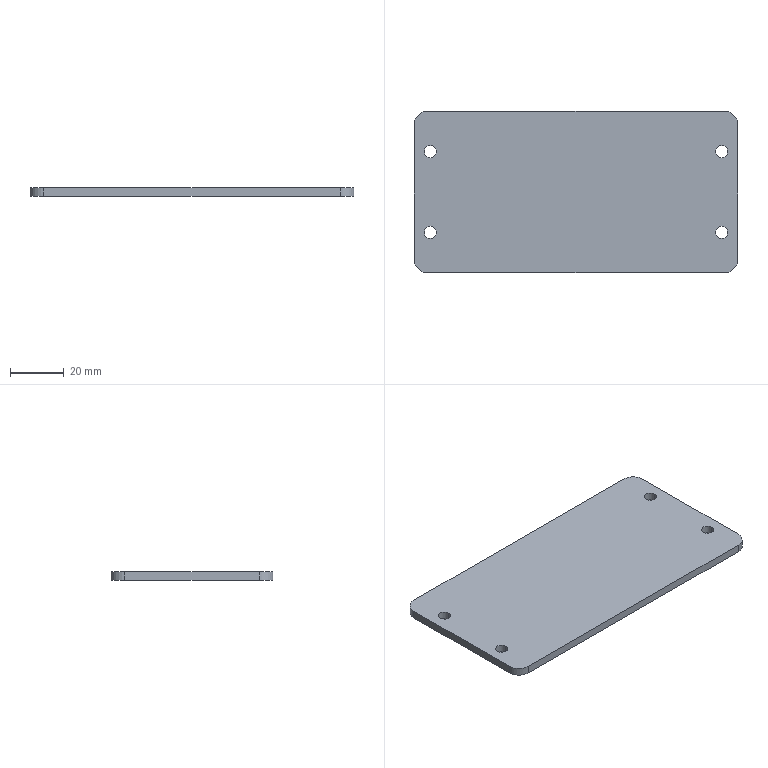Part | STEP file | 03-24 side guard plate | 1 solid | 18 faces | box 120 x 60 x 3 mm | volume 21345 mm3 | cylinder 12 | plane 6 | commonest cylinder face diameters 4.5 x8 10 x4
STEP:
#1=CARTESIAN_POINT('',(51.75,-15.,0.));
#2=VERTEX_POINT('',#1);
#3=CARTESIAN_POINT('',(56.25,-15.,0.));
#4=VERTEX_POINT('',#3);
#5=CARTESIAN_POINT('',(54.,-15.,0.));
#6=DIRECTION('',(0.,0.,1.));
#7=DIRECTION('',(1.,0.,0.));
#8=AXIS2_PLACEMENT_3D('',#5,#6,#7);
#9=CIRCLE('',#8,2.25);
#10=EDGE_CURVE('',#2,#4,#9,.T.);
#11=ORIENTED_EDGE('',*,*,#10,.F.);
#12=CARTESIAN_POINT('',(51.75,-15.,3.));
#13=VERTEX_POINT('',#12);
#14=CARTESIAN_POINT('',(51.75,-15.,-2.));
#15=DIRECTION('',(0.,0.,1.));
#16=VECTOR('',#15,1000.);
#17=LINE('',#14,#16);
#18=EDGE_CURVE('',#2,#13,#17,.T.);
#19=ORIENTED_EDGE('',*,*,#18,.T.);
#20=CARTESIAN_POINT('',(56.25,-15.,3.));
#21=VERTEX_POINT('',#20);
#22=CARTESIAN_POINT('',(54.,-15.,3.));
#23=DIRECTION('',(0.,0.,1.));
#24=DIRECTION('',(-1.,0.,0.));
#25=AXIS2_PLACEMENT_3D('',#22,#23,#24);
#26=CIRCLE('',#25,2.25);
#27=EDGE_CURVE('',#13,#21,#26,.T.);
#28=ORIENTED_EDGE('',*,*,#27,.T.);
#29=CARTESIAN_POINT('',(56.25,-15.,-2.));
#30=DIRECTION('',(0.,0.,1.));
#31=VECTOR('',#30,1000.);
#32=LINE('',#29,#31);
#33=EDGE_CURVE('',#4,#21,#32,.T.);
#34=ORIENTED_EDGE('',*,*,#33,.F.);
#35=EDGE_LOOP('',(#11,#19,#28,#34));
#36=FACE_OUTER_BOUND('',#35,.T.);
#37=CARTESIAN_POINT('',(54.,-15.,-2.));
#38=DIRECTION('',(0.,0.,1.));
#39=DIRECTION('',(1.,0.,0.));
#40=AXIS2_PLACEMENT_3D('',#37,#38,#39);
#41=CYLINDRICAL_SURFACE('',#40,2.25);
#42=ADVANCED_FACE('',(#36),#41,.F.);
#43=CARTESIAN_POINT('',(-56.25,15.,0.));
#44=VERTEX_POINT('',#43);
#45=CARTESIAN_POINT('',(-51.75,15.,0.));
#46=VERTEX_POINT('',#45);
#47=CARTESIAN_POINT('',(-54.,15.,0.));
#48=DIRECTION('',(0.,0.,1.));
#49=DIRECTION('',(1.,0.,0.));
#50=AXIS2_PLACEMENT_3D('',#47,#48,#49);
#51=CIRCLE('',#50,2.25);
#52=EDGE_CURVE('',#44,#46,#51,.T.);
#53=ORIENTED_EDGE('',*,*,#52,.F.);
#54=CARTESIAN_POINT('',(-56.25,15.,3.));
#55=VERTEX_POINT('',#54);
#56=CARTESIAN_POINT('',(-56.25,15.,-2.));
#57=DIRECTION('',(0.,0.,1.));
#58=VECTOR('',#57,1000.);
#59=LINE('',#56,#58);
#60=EDGE_CURVE('',#44,#55,#59,.T.);
#61=ORIENTED_EDGE('',*,*,#60,.T.);
#62=CARTESIAN_POINT('',(-51.75,15.,3.));
#63=VERTEX_POINT('',#62);
#64=CARTESIAN_POINT('',(-54.,15.,3.));
#65=DIRECTION('',(0.,0.,1.));
#66=DIRECTION('',(-1.,0.,0.));
#67=AXIS2_PLACEMENT_3D('',#64,#65,#66);
#68=CIRCLE('',#67,2.25);
#69=EDGE_CURVE('',#55,#63,#68,.T.);
#70=ORIENTED_EDGE('',*,*,#69,.T.);
#71=CARTESIAN_POINT('',(-51.75,15.,-2.));
#72=DIRECTION('',(0.,0.,1.));
#73=VECTOR('',#72,1000.);
#74=LINE('',#71,#73);
#75=EDGE_CURVE('',#46,#63,#74,.T.);
#76=ORIENTED_EDGE('',*,*,#75,.F.);
#77=EDGE_LOOP('',(#53,#61,#70,#76));
#78=FACE_OUTER_BOUND('',#77,.T.);
#79=CARTESIAN_POINT('',(-54.,15.,-2.));
#80=DIRECTION('',(0.,0.,1.));
#81=DIRECTION('',(1.,0.,0.));
#82=AXIS2_PLACEMENT_3D('',#79,#80,#81);
#83=CYLINDRICAL_SURFACE('',#82,2.25);
#84=ADVANCED_FACE('',(#78),#83,.F.);
#85=CARTESIAN_POINT('',(-56.25,-15.,0.));
#86=VERTEX_POINT('',#85);
#87=CARTESIAN_POINT('',(-51.75,-15.,0.));
#88=VERTEX_POINT('',#87);
#89=CARTESIAN_POINT('',(-54.,-15.,0.));
#90=DIRECTION('',(0.,0.,1.));
#91=DIRECTION('',(1.,0.,0.));
#92=AXIS2_PLACEMENT_3D('',#89,#90,#91);
#93=CIRCLE('',#92,2.25);
#94=EDGE_CURVE('',#86,#88,#93,.T.);
#95=ORIENTED_EDGE('',*,*,#94,.F.);
#96=CARTESIAN_POINT('',(-56.25,-15.,3.));
#97=VERTEX_POINT('',#96);
#98=CARTESIAN_POINT('',(-56.25,-15.,-2.));
#99=DIRECTION('',(0.,0.,1.));
#100=VECTOR('',#99,1000.);
#101=LINE('',#98,#100);
#102=EDGE_CURVE('',#86,#97,#101,.T.);
#103=ORIENTED_EDGE('',*,*,#102,.T.);
#104=CARTESIAN_POINT('',(-51.75,-15.,3.));
#105=VERTEX_POINT('',#104);
#106=CARTESIAN_POINT('',(-54.,-15.,3.));
#107=DIRECTION('',(0.,0.,1.));
#108=DIRECTION('',(1.,0.,0.));
#109=AXIS2_PLACEMENT_3D('',#106,#107,#108);
#110=CIRCLE('',#109,2.25);
#111=EDGE_CURVE('',#97,#105,#110,.T.);
#112=ORIENTED_EDGE('',*,*,#111,.T.);
#113=CARTESIAN_POINT('',(-51.75,-15.,-2.));
#114=DIRECTION('',(0.,0.,1.));
#115=VECTOR('',#114,1000.);
#116=LINE('',#113,#115);
#117=EDGE_CURVE('',#88,#105,#116,.T.);
#118=ORIENTED_EDGE('',*,*,#117,.F.);
#119=EDGE_LOOP('',(#95,#103,#112,#118));
#120=FACE_OUTER_BOUND('',#119,.T.);
#121=CARTESIAN_POINT('',(-54.,-15.,-2.));
#122=DIRECTION('',(0.,0.,1.));
#123=DIRECTION('',(1.,0.,0.));
#124=AXIS2_PLACEMENT_3D('',#121,#122,#123);
#125=CYLINDRICAL_SURFACE('',#124,2.25);
#126=ADVANCED_FACE('',(#120),#125,.F.);
#127=CARTESIAN_POINT('',(51.75,15.,0.));
#128=VERTEX_POINT('',#127);
#129=CARTESIAN_POINT('',(56.25,15.,0.));
#130=VERTEX_POINT('',#129);
#131=CARTESIAN_POINT('',(54.,15.,0.));
#132=DIRECTION('',(0.,0.,1.));
#133=DIRECTION('',(1.,0.,0.));
#134=AXIS2_PLACEMENT_3D('',#131,#132,#133);
#135=CIRCLE('',#134,2.25);
#136=EDGE_CURVE('',#128,#130,#135,.T.);
#137=ORIENTED_EDGE('',*,*,#136,.F.);
#138=CARTESIAN_POINT('',(51.75,15.,3.));
#139=VERTEX_POINT('',#138);
#140=CARTESIAN_POINT('',(51.75,15.,-2.));
#141=DIRECTION('',(0.,0.,1.));
#142=VECTOR('',#141,1000.);
#143=LINE('',#140,#142);
#144=EDGE_CURVE('',#128,#139,#143,.T.);
#145=ORIENTED_EDGE('',*,*,#144,.T.);
#146=CARTESIAN_POINT('',(56.25,15.,3.));
#147=VERTEX_POINT('',#146);
#148=CARTESIAN_POINT('',(54.,15.,3.));
#149=DIRECTION('',(0.,0.,1.));
#150=DIRECTION('',(1.,0.,0.));
#151=AXIS2_PLACEMENT_3D('',#148,#149,#150);
#152=CIRCLE('',#151,2.25);
#153=EDGE_CURVE('',#139,#147,#152,.T.);
#154=ORIENTED_EDGE('',*,*,#153,.T.);
#155=CARTESIAN_POINT('',(56.25,15.,-2.));
#156=DIRECTION('',(0.,0.,1.));
#157=VECTOR('',#156,1000.);
#158=LINE('',#155,#157);
#159=EDGE_CURVE('',#130,#147,#158,.T.);
#160=ORIENTED_EDGE('',*,*,#159,.F.);
#161=EDGE_LOOP('',(#137,#145,#154,#160));
#162=FACE_OUTER_BOUND('',#161,.T.);
#163=CARTESIAN_POINT('',(54.,15.,-2.));
#164=DIRECTION('',(0.,0.,1.));
#165=DIRECTION('',(1.,0.,0.));
#166=AXIS2_PLACEMENT_3D('',#163,#164,#165);
#167=CYLINDRICAL_SURFACE('',#166,2.25);
#168=ADVANCED_FACE('',(#162),#167,.F.);
#169=CARTESIAN_POINT('',(60.,-25.,3.));
#170=VERTEX_POINT('',#169);
#171=CARTESIAN_POINT('',(60.,25.,3.));
#172=VERTEX_POINT('',#171);
#173=CARTESIAN_POINT('',(60.,30.,3.));
#174=DIRECTION('',(0.,1.,0.));
#175=VECTOR('',#174,1000.);
#176=LINE('',#173,#175);
#177=EDGE_CURVE('',#170,#172,#176,.T.);
#178=ORIENTED_EDGE('',*,*,#177,.F.);
#179=CARTESIAN_POINT('',(60.,-25.,0.));
#180=VERTEX_POINT('',#179);
#181=CARTESIAN_POINT('',(60.,-25.,3.));
#182=DIRECTION('',(0.,0.,-1.));
#183=VECTOR('',#182,1000.);
#184=LINE('',#181,#183);
#185=EDGE_CURVE('',#170,#180,#184,.T.);
#186=ORIENTED_EDGE('',*,*,#185,.T.);
#187=CARTESIAN_POINT('',(60.,25.,0.));
#188=VERTEX_POINT('',#187);
#189=CARTESIAN_POINT('',(60.,30.,0.));
#190=DIRECTION('',(0.,1.,0.));
#191=VECTOR('',#190,1000.);
#192=LINE('',#189,#191);
#193=EDGE_CURVE('',#180,#188,#192,.T.);
#194=ORIENTED_EDGE('',*,*,#193,.T.);
#195=CARTESIAN_POINT('',(60.,25.,3.));
#196=DIRECTION('',(0.,0.,1.));
#197=VECTOR('',#196,1000.);
#198=LINE('',#195,#197);
#199=EDGE_CURVE('',#188,#172,#198,.T.);
#200=ORIENTED_EDGE('',*,*,#199,.T.);
#201=EDGE_LOOP('',(#178,#186,#194,#200));
#202=FACE_OUTER_BOUND('',#201,.T.);
#203=CARTESIAN_POINT('',(60.,30.,3.));
#204=DIRECTION('',(-1.,0.,0.));
#205=DIRECTION('',(0.,-1.,0.));
#206=AXIS2_PLACEMENT_3D('',#203,#204,#205);
#207=PLANE('',#206);
#208=ADVANCED_FACE('',(#202),#207,.F.);
#209=CARTESIAN_POINT('',(55.,30.,3.));
#210=VERTEX_POINT('',#209);
#211=CARTESIAN_POINT('',(-55.,30.,3.));
#212=VERTEX_POINT('',#211);
#213=CARTESIAN_POINT('',(-60.,30.,3.));
#214=DIRECTION('',(-1.,0.,0.));
#215=VECTOR('',#214,1000.);
#216=LINE('',#213,#215);
#217=EDGE_CURVE('',#210,#212,#216,.T.);
#218=ORIENTED_EDGE('',*,*,#217,.F.);
#219=CARTESIAN_POINT('',(55.,30.,0.));
#220=VERTEX_POINT('',#219);
#221=CARTESIAN_POINT('',(55.,30.,3.));
#222=DIRECTION('',(0.,0.,-1.));
#223=VECTOR('',#222,1000.);
#224=LINE('',#221,#223);
#225=EDGE_CURVE('',#210,#220,#224,.T.);
#226=ORIENTED_EDGE('',*,*,#225,.T.);
#227=CARTESIAN_POINT('',(-55.,30.,0.));
#228=VERTEX_POINT('',#227);
#229=CARTESIAN_POINT('',(-60.,30.,0.));
#230=DIRECTION('',(-1.,0.,0.));
#231=VECTOR('',#230,1000.);
#232=LINE('',#229,#231);
#233=EDGE_CURVE('',#220,#228,#232,.T.);
#234=ORIENTED_EDGE('',*,*,#233,.T.);
#235=CARTESIAN_POINT('',(-55.,30.,3.));
#236=DIRECTION('',(0.,0.,1.));
#237=VECTOR('',#236,1000.);
#238=LINE('',#235,#237);
#239=EDGE_CURVE('',#228,#212,#238,.T.);
#240=ORIENTED_EDGE('',*,*,#239,.T.);
#241=EDGE_LOOP('',(#218,#226,#234,#240));
#242=FACE_OUTER_BOUND('',#241,.T.);
#243=CARTESIAN_POINT('',(-60.,30.,3.));
#244=DIRECTION('',(0.,-1.,0.));
#245=DIRECTION('',(0.,0.,-1.));
#246=AXIS2_PLACEMENT_3D('',#243,#244,#245);
#247=PLANE('',#246);
#248=ADVANCED_FACE('',(#242),#247,.F.);
#249=CARTESIAN_POINT('',(-60.,25.,0.));
#250=VERTEX_POINT('',#249);
#251=CARTESIAN_POINT('',(-60.,-25.,0.));
#252=VERTEX_POINT('',#251);
#253=CARTESIAN_POINT('',(-60.,30.,0.));
#254=DIRECTION('',(0.,-1.,0.));
#255=VECTOR('',#254,1000.);
#256=LINE('',#253,#255);
#257=EDGE_CURVE('',#250,#252,#256,.T.);
#258=ORIENTED_EDGE('',*,*,#257,.T.);
#259=CARTESIAN_POINT('',(-60.,-25.,3.));
#260=VERTEX_POINT('',#259);
#261=CARTESIAN_POINT('',(-60.,-25.,3.));
#262=DIRECTION('',(0.,0.,1.));
#263=VECTOR('',#262,1000.);
#264=LINE('',#261,#263);
#265=EDGE_CURVE('',#252,#260,#264,.T.);
#266=ORIENTED_EDGE('',*,*,#265,.T.);
#267=CARTESIAN_POINT('',(-60.,25.,3.));
#268=VERTEX_POINT('',#267);
#269=CARTESIAN_POINT('',(-60.,30.,3.));
#270=DIRECTION('',(0.,-1.,0.));
#271=VECTOR('',#270,1000.);
#272=LINE('',#269,#271);
#273=EDGE_CURVE('',#268,#260,#272,.T.);
#274=ORIENTED_EDGE('',*,*,#273,.F.);
#275=CARTESIAN_POINT('',(-60.,25.,3.));
#276=DIRECTION('',(0.,0.,-1.));
#277=VECTOR('',#276,1000.);
#278=LINE('',#275,#277);
#279=EDGE_CURVE('',#268,#250,#278,.T.);
#280=ORIENTED_EDGE('',*,*,#279,.T.);
#281=EDGE_LOOP('',(#258,#266,#274,#280));
#282=FACE_OUTER_BOUND('',#281,.T.);
#283=CARTESIAN_POINT('',(-60.,30.,3.));
#284=DIRECTION('',(1.,0.,0.));
#285=DIRECTION('',(0.,1.,0.));
#286=AXIS2_PLACEMENT_3D('',#283,#284,#285);
#287=PLANE('',#286);
#288=ADVANCED_FACE('',(#282),#287,.F.);
#289=CARTESIAN_POINT('',(-55.,-30.,0.));
#290=VERTEX_POINT('',#289);
#291=CARTESIAN_POINT('',(55.,-30.,0.));
#292=VERTEX_POINT('',#291);
#293=CARTESIAN_POINT('',(-60.,-30.,0.));
#294=DIRECTION('',(1.,0.,0.));
#295=VECTOR('',#294,1000.);
#296=LINE('',#293,#295);
#297=EDGE_CURVE('',#290,#292,#296,.T.);
#298=ORIENTED_EDGE('',*,*,#297,.T.);
#299=CARTESIAN_POINT('',(55.,-30.,3.));
#300=VERTEX_POINT('',#299);
#301=CARTESIAN_POINT('',(55.,-30.,3.));
#302=DIRECTION('',(0.,0.,1.));
#303=VECTOR('',#302,1000.);
#304=LINE('',#301,#303);
#305=EDGE_CURVE('',#292,#300,#304,.T.);
#306=ORIENTED_EDGE('',*,*,#305,.T.);
#307=CARTESIAN_POINT('',(-55.,-30.,3.));
#308=VERTEX_POINT('',#307);
#309=CARTESIAN_POINT('',(-60.,-30.,3.));
#310=DIRECTION('',(1.,0.,0.));
#311=VECTOR('',#310,1000.);
#312=LINE('',#309,#311);
#313=EDGE_CURVE('',#308,#300,#312,.T.);
#314=ORIENTED_EDGE('',*,*,#313,.F.);
#315=CARTESIAN_POINT('',(-55.,-30.,3.));
#316=DIRECTION('',(0.,0.,-1.));
#317=VECTOR('',#316,1000.);
#318=LINE('',#315,#317);
#319=EDGE_CURVE('',#308,#290,#318,.T.);
#320=ORIENTED_EDGE('',*,*,#319,.T.);
#321=EDGE_LOOP('',(#298,#306,#314,#320));
#322=FACE_OUTER_BOUND('',#321,.T.);
#323=CARTESIAN_POINT('',(-60.,-30.,3.));
#324=DIRECTION('',(0.,1.,0.));
#325=DIRECTION('',(0.,0.,1.));
#326=AXIS2_PLACEMENT_3D('',#323,#324,#325);
#327=PLANE('',#326);
#328=ADVANCED_FACE('',(#322),#327,.F.);
#329=CARTESIAN_POINT('',(54.,-15.,3.));
#330=DIRECTION('',(0.,0.,1.));
#331=DIRECTION('',(-1.,0.,0.));
#332=AXIS2_PLACEMENT_3D('',#329,#330,#331);
#333=CIRCLE('',#332,2.25);
#334=EDGE_CURVE('',#21,#13,#333,.T.);
#335=ORIENTED_EDGE('',*,*,#334,.F.);
#336=ORIENTED_EDGE('',*,*,#27,.F.);
#337=EDGE_LOOP('',(#335,#336));
#338=FACE_BOUND('',#337,.T.);
#339=CARTESIAN_POINT('',(-54.,15.,3.));
#340=DIRECTION('',(0.,0.,1.));
#341=DIRECTION('',(-1.,0.,0.));
#342=AXIS2_PLACEMENT_3D('',#339,#340,#341);
#343=CIRCLE('',#342,2.25);
#344=EDGE_CURVE('',#63,#55,#343,.T.);
#345=ORIENTED_EDGE('',*,*,#344,.F.);
#346=ORIENTED_EDGE('',*,*,#69,.F.);
#347=EDGE_LOOP('',(#345,#346));
#348=FACE_BOUND('',#347,.T.);
#349=CARTESIAN_POINT('',(-54.,-15.,3.));
#350=DIRECTION('',(0.,0.,1.));
#351=DIRECTION('',(1.,0.,0.));
#352=AXIS2_PLACEMENT_3D('',#349,#350,#351);
#353=CIRCLE('',#352,2.25);
#354=EDGE_CURVE('',#105,#97,#353,.T.);
#355=ORIENTED_EDGE('',*,*,#354,.F.);
#356=ORIENTED_EDGE('',*,*,#111,.F.);
#357=EDGE_LOOP('',(#355,#356));
#358=FACE_BOUND('',#357,.T.);
#359=CARTESIAN_POINT('',(54.,15.,3.));
#360=DIRECTION('',(0.,0.,1.));
#361=DIRECTION('',(1.,0.,0.));
#362=AXIS2_PLACEMENT_3D('',#359,#360,#361);
#363=CIRCLE('',#362,2.25);
#364=EDGE_CURVE('',#147,#139,#363,.T.);
#365=ORIENTED_EDGE('',*,*,#364,.F.);
#366=ORIENTED_EDGE('',*,*,#153,.F.);
#367=EDGE_LOOP('',(#365,#366));
#368=FACE_BOUND('',#367,.T.);
#369=ORIENTED_EDGE('',*,*,#313,.T.);
#370=CARTESIAN_POINT('',(55.,-25.,3.));
#371=DIRECTION('',(0.,0.,1.));
#372=DIRECTION('',(1.,0.,0.));
#373=AXIS2_PLACEMENT_3D('',#370,#371,#372);
#374=CIRCLE('',#373,5.);
#375=EDGE_CURVE('',#300,#170,#374,.T.);
#376=ORIENTED_EDGE('',*,*,#375,.T.);
#377=ORIENTED_EDGE('',*,*,#177,.T.);
#378=CARTESIAN_POINT('',(55.,25.,3.));
#379=DIRECTION('',(0.,0.,1.));
#380=DIRECTION('',(1.,0.,0.));
#381=AXIS2_PLACEMENT_3D('',#378,#379,#380);
#382=CIRCLE('',#381,5.);
#383=EDGE_CURVE('',#172,#210,#382,.T.);
#384=ORIENTED_EDGE('',*,*,#383,.T.);
#385=ORIENTED_EDGE('',*,*,#217,.T.);
#386=CARTESIAN_POINT('',(-55.,25.,3.));
#387=DIRECTION('',(0.,0.,1.));
#388=DIRECTION('',(1.,0.,0.));
#389=AXIS2_PLACEMENT_3D('',#386,#387,#388);
#390=CIRCLE('',#389,5.);
#391=EDGE_CURVE('',#212,#268,#390,.T.);
#392=ORIENTED_EDGE('',*,*,#391,.T.);
#393=ORIENTED_EDGE('',*,*,#273,.T.);
#394=CARTESIAN_POINT('',(-55.,-25.,3.));
#395=DIRECTION('',(0.,0.,1.));
#396=DIRECTION('',(1.,0.,0.));
#397=AXIS2_PLACEMENT_3D('',#394,#395,#396);
#398=CIRCLE('',#397,5.);
#399=EDGE_CURVE('',#260,#308,#398,.T.);
#400=ORIENTED_EDGE('',*,*,#399,.T.);
#401=EDGE_LOOP('',(#369,#376,#377,#384,#385,#392,#393,#400));
#402=FACE_OUTER_BOUND('',#401,.T.);
#403=CARTESIAN_POINT('',(60.,-30.,3.));
#404=DIRECTION('',(0.,0.,1.));
#405=DIRECTION('',(1.,0.,0.));
#406=AXIS2_PLACEMENT_3D('',#403,#404,#405);
#407=PLANE('',#406);
#408=ADVANCED_FACE('',(#338,#348,#358,#368,#402),#407,.T.);
#409=CARTESIAN_POINT('',(54.,-15.,0.));
#410=DIRECTION('',(0.,0.,1.));
#411=DIRECTION('',(1.,0.,0.));
#412=AXIS2_PLACEMENT_3D('',#409,#410,#411);
#413=CIRCLE('',#412,2.25);
#414=EDGE_CURVE('',#4,#2,#413,.T.);
#415=ORIENTED_EDGE('',*,*,#414,.T.);
#416=ORIENTED_EDGE('',*,*,#10,.T.);
#417=EDGE_LOOP('',(#415,#416));
#418=FACE_BOUND('',#417,.T.);
#419=CARTESIAN_POINT('',(-54.,15.,0.));
#420=DIRECTION('',(0.,0.,1.));
#421=DIRECTION('',(1.,0.,0.));
#422=AXIS2_PLACEMENT_3D('',#419,#420,#421);
#423=CIRCLE('',#422,2.25);
#424=EDGE_CURVE('',#46,#44,#423,.T.);
#425=ORIENTED_EDGE('',*,*,#424,.T.);
#426=ORIENTED_EDGE('',*,*,#52,.T.);
#427=EDGE_LOOP('',(#425,#426));
#428=FACE_BOUND('',#427,.T.);
#429=CARTESIAN_POINT('',(-54.,-15.,0.));
#430=DIRECTION('',(0.,0.,1.));
#431=DIRECTION('',(1.,0.,0.));
#432=AXIS2_PLACEMENT_3D('',#429,#430,#431);
#433=CIRCLE('',#432,2.25);
#434=EDGE_CURVE('',#88,#86,#433,.T.);
#435=ORIENTED_EDGE('',*,*,#434,.T.);
#436=ORIENTED_EDGE('',*,*,#94,.T.);
#437=EDGE_LOOP('',(#435,#436));
#438=FACE_BOUND('',#437,.T.);
#439=CARTESIAN_POINT('',(54.,15.,0.));
#440=DIRECTION('',(0.,0.,1.));
#441=DIRECTION('',(1.,0.,0.));
#442=AXIS2_PLACEMENT_3D('',#439,#440,#441);
#443=CIRCLE('',#442,2.25);
#444=EDGE_CURVE('',#130,#128,#443,.T.);
#445=ORIENTED_EDGE('',*,*,#444,.T.);
#446=ORIENTED_EDGE('',*,*,#136,.T.);
#447=EDGE_LOOP('',(#445,#446));
#448=FACE_BOUND('',#447,.T.);
#449=ORIENTED_EDGE('',*,*,#193,.F.);
#450=CARTESIAN_POINT('',(55.,-25.,0.));
#451=DIRECTION('',(0.,0.,-1.));
#452=DIRECTION('',(1.,0.,0.));
#453=AXIS2_PLACEMENT_3D('',#450,#451,#452);
#454=CIRCLE('',#453,5.);
#455=EDGE_CURVE('',#180,#292,#454,.T.);
#456=ORIENTED_EDGE('',*,*,#455,.T.);
#457=ORIENTED_EDGE('',*,*,#297,.F.);
#458=CARTESIAN_POINT('',(-55.,-25.,0.));
#459=DIRECTION('',(0.,0.,-1.));
#460=DIRECTION('',(1.,0.,0.));
#461=AXIS2_PLACEMENT_3D('',#458,#459,#460);
#462=CIRCLE('',#461,5.);
#463=EDGE_CURVE('',#290,#252,#462,.T.);
#464=ORIENTED_EDGE('',*,*,#463,.T.);
#465=ORIENTED_EDGE('',*,*,#257,.F.);
#466=CARTESIAN_POINT('',(-55.,25.,0.));
#467=DIRECTION('',(0.,0.,-1.));
#468=DIRECTION('',(1.,0.,0.));
#469=AXIS2_PLACEMENT_3D('',#466,#467,#468);
#470=CIRCLE('',#469,5.);
#471=EDGE_CURVE('',#250,#228,#470,.T.);
#472=ORIENTED_EDGE('',*,*,#471,.T.);
#473=ORIENTED_EDGE('',*,*,#233,.F.);
#474=CARTESIAN_POINT('',(55.,25.,0.));
#475=DIRECTION('',(0.,0.,-1.));
#476=DIRECTION('',(1.,0.,0.));
#477=AXIS2_PLACEMENT_3D('',#474,#475,#476);
#478=CIRCLE('',#477,5.);
#479=EDGE_CURVE('',#220,#188,#478,.T.);
#480=ORIENTED_EDGE('',*,*,#479,.T.);
#481=EDGE_LOOP('',(#449,#456,#457,#464,#465,#472,#473,#480));
#482=FACE_OUTER_BOUND('',#481,.T.);
#483=CARTESIAN_POINT('',(60.,-30.,0.));
#484=DIRECTION('',(0.,0.,1.));
#485=DIRECTION('',(1.,0.,0.));
#486=AXIS2_PLACEMENT_3D('',#483,#484,#485);
#487=PLANE('',#486);
#488=ADVANCED_FACE('',(#418,#428,#438,#448,#482),#487,.F.);
#489=ORIENTED_EDGE('',*,*,#375,.F.);
#490=ORIENTED_EDGE('',*,*,#305,.F.);
#491=ORIENTED_EDGE('',*,*,#455,.F.);
#492=ORIENTED_EDGE('',*,*,#185,.F.);
#493=EDGE_LOOP('',(#489,#490,#491,#492));
#494=FACE_OUTER_BOUND('',#493,.T.);
#495=CARTESIAN_POINT('',(55.,-25.,3.));
#496=DIRECTION('',(0.,0.,-1.));
#497=DIRECTION('',(-1.,0.,0.));
#498=AXIS2_PLACEMENT_3D('',#495,#496,#497);
#499=CYLINDRICAL_SURFACE('',#498,5.);
#500=ADVANCED_FACE('',(#494),#499,.T.);
#501=ORIENTED_EDGE('',*,*,#383,.F.);
#502=ORIENTED_EDGE('',*,*,#199,.F.);
#503=ORIENTED_EDGE('',*,*,#479,.F.);
#504=ORIENTED_EDGE('',*,*,#225,.F.);
#505=EDGE_LOOP('',(#501,#502,#503,#504));
#506=FACE_OUTER_BOUND('',#505,.T.);
#507=CARTESIAN_POINT('',(55.,25.,3.));
#508=DIRECTION('',(0.,0.,-1.));
#509=DIRECTION('',(-1.,0.,0.));
#510=AXIS2_PLACEMENT_3D('',#507,#508,#509);
#511=CYLINDRICAL_SURFACE('',#510,5.);
#512=ADVANCED_FACE('',(#506),#511,.T.);
#513=ORIENTED_EDGE('',*,*,#399,.F.);
#514=ORIENTED_EDGE('',*,*,#265,.F.);
#515=ORIENTED_EDGE('',*,*,#463,.F.);
#516=ORIENTED_EDGE('',*,*,#319,.F.);
#517=EDGE_LOOP('',(#513,#514,#515,#516));
#518=FACE_OUTER_BOUND('',#517,.T.);
#519=CARTESIAN_POINT('',(-55.,-25.,3.));
#520=DIRECTION('',(0.,0.,-1.));
#521=DIRECTION('',(-1.,0.,0.));
#522=AXIS2_PLACEMENT_3D('',#519,#520,#521);
#523=CYLINDRICAL_SURFACE('',#522,5.);
#524=ADVANCED_FACE('',(#518),#523,.T.);
#525=ORIENTED_EDGE('',*,*,#391,.F.);
#526=ORIENTED_EDGE('',*,*,#239,.F.);
#527=ORIENTED_EDGE('',*,*,#471,.F.);
#528=ORIENTED_EDGE('',*,*,#279,.F.);
#529=EDGE_LOOP('',(#525,#526,#527,#528));
#530=FACE_OUTER_BOUND('',#529,.T.);
#531=CARTESIAN_POINT('',(-55.,25.,3.));
#532=DIRECTION('',(0.,0.,-1.));
#533=DIRECTION('',(-1.,0.,0.));
#534=AXIS2_PLACEMENT_3D('',#531,#532,#533);
#535=CYLINDRICAL_SURFACE('',#534,5.);
#536=ADVANCED_FACE('',(#530),#535,.T.);
#537=ORIENTED_EDGE('',*,*,#144,.F.);
#538=ORIENTED_EDGE('',*,*,#444,.F.);
#539=ORIENTED_EDGE('',*,*,#159,.T.);
#540=ORIENTED_EDGE('',*,*,#364,.T.);
#541=EDGE_LOOP('',(#537,#538,#539,#540));
#542=FACE_OUTER_BOUND('',#541,.T.);
#543=CARTESIAN_POINT('',(54.,15.,-2.));
#544=DIRECTION('',(0.,0.,1.));
#545=DIRECTION('',(1.,0.,0.));
#546=AXIS2_PLACEMENT_3D('',#543,#544,#545);
#547=CYLINDRICAL_SURFACE('',#546,2.25);
#548=ADVANCED_FACE('',(#542),#547,.F.);
#549=ORIENTED_EDGE('',*,*,#102,.F.);
#550=ORIENTED_EDGE('',*,*,#434,.F.);
#551=ORIENTED_EDGE('',*,*,#117,.T.);
#552=ORIENTED_EDGE('',*,*,#354,.T.);
#553=EDGE_LOOP('',(#549,#550,#551,#552));
#554=FACE_OUTER_BOUND('',#553,.T.);
#555=CARTESIAN_POINT('',(-54.,-15.,-2.));
#556=DIRECTION('',(0.,0.,1.));
#557=DIRECTION('',(1.,0.,0.));
#558=AXIS2_PLACEMENT_3D('',#555,#556,#557);
#559=CYLINDRICAL_SURFACE('',#558,2.25);
#560=ADVANCED_FACE('',(#554),#559,.F.);
#561=ORIENTED_EDGE('',*,*,#60,.F.);
#562=ORIENTED_EDGE('',*,*,#424,.F.);
#563=ORIENTED_EDGE('',*,*,#75,.T.);
#564=ORIENTED_EDGE('',*,*,#344,.T.);
#565=EDGE_LOOP('',(#561,#562,#563,#564));
#566=FACE_OUTER_BOUND('',#565,.T.);
#567=CARTESIAN_POINT('',(-54.,15.,-2.));
#568=DIRECTION('',(0.,0.,1.));
#569=DIRECTION('',(1.,0.,0.));
#570=AXIS2_PLACEMENT_3D('',#567,#568,#569);
#571=CYLINDRICAL_SURFACE('',#570,2.25);
#572=ADVANCED_FACE('',(#566),#571,.F.);
#573=ORIENTED_EDGE('',*,*,#18,.F.);
#574=ORIENTED_EDGE('',*,*,#414,.F.);
#575=ORIENTED_EDGE('',*,*,#33,.T.);
#576=ORIENTED_EDGE('',*,*,#334,.T.);
#577=EDGE_LOOP('',(#573,#574,#575,#576));
#578=FACE_OUTER_BOUND('',#577,.T.);
#579=CARTESIAN_POINT('',(54.,-15.,-2.));
#580=DIRECTION('',(0.,0.,1.));
#581=DIRECTION('',(1.,0.,0.));
#582=AXIS2_PLACEMENT_3D('',#579,#580,#581);
#583=CYLINDRICAL_SURFACE('',#582,2.25);
#584=ADVANCED_FACE('',(#578),#583,.F.);
#585=CLOSED_SHELL('',(#42,#84,#126,#168,#208,#248,#288,#328,#408,#488,#500,#512,#524,#536,#548,#560,#572,#584));
#586=MANIFOLD_SOLID_BREP('',#585);
#587=CARTESIAN_POINT('',(0.,0.,0.));
#588=DIRECTION('',(0.,0.,1.));
#589=DIRECTION('',(1.,0.,0.));
#590=AXIS2_PLACEMENT_3D('',#587,#588,#589);
#591=(LENGTH_UNIT()NAMED_UNIT(*)SI_UNIT(.MILLI.,.METRE.));
#592=UNCERTAINTY_MEASURE_WITH_UNIT(LENGTH_MEASURE(0.00001),#591,'','');
#593=(NAMED_UNIT(*)PLANE_ANGLE_UNIT()SI_UNIT($,.RADIAN.));
#594=(NAMED_UNIT(*)SI_UNIT($,.STERADIAN.)SOLID_ANGLE_UNIT());
#595=(GEOMETRIC_REPRESENTATION_CONTEXT(3)GLOBAL_UNCERTAINTY_ASSIGNED_CONTEXT((#592))GLOBAL_UNIT_ASSIGNED_CONTEXT((#591,#593,#594))REPRESENTATION_CONTEXT('',''));
#596=ADVANCED_BREP_SHAPE_REPRESENTATION('',(#586,#590),#595);